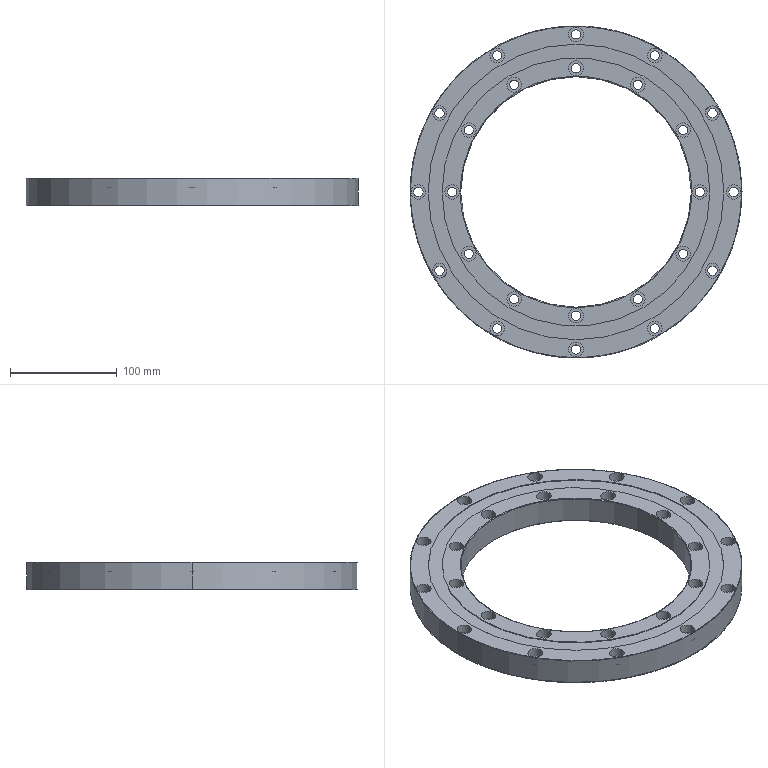Part | STEP file | EFXU21626 | 1 solid | 149 faces | box 311 x 311 x 25.4 mm | volume 912678 mm3 | cylinder 110 | plane 31 | spline 8 | commonest cylinder face diameters 8.7 x48 13.7 x48 251 x4 215.9 x2 263.4 x2 264.6 x2